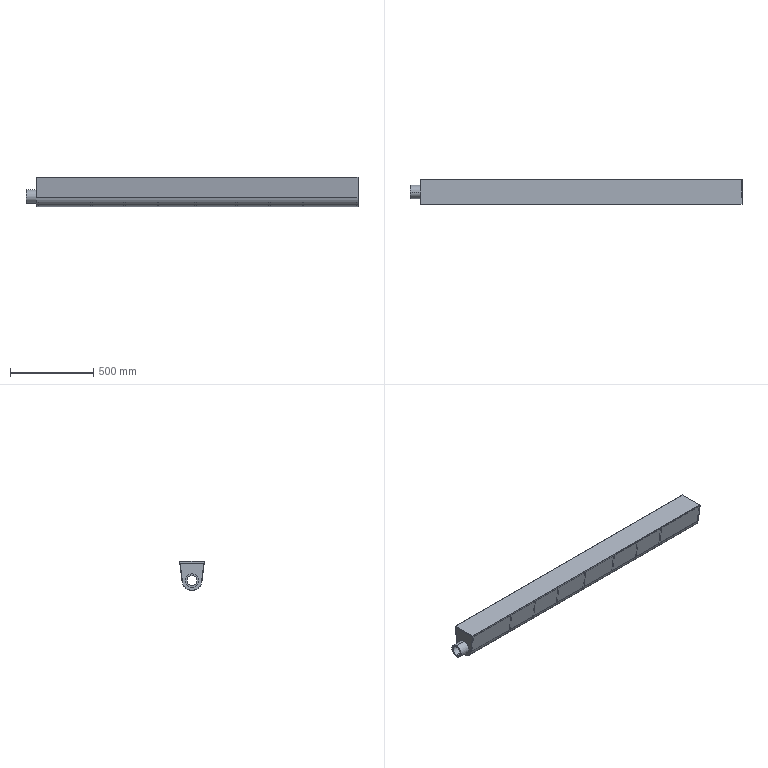Part | SolidWorks | features MirrorStock 1 | 12 solids | 100 faces | box 1995 x 150 x 175 mm | volume 10047262 mm3 | plane 61 | cylinder 39 | commonest cylinder face diameters 80 x20 116 x11 10 x4 60 x2 120 x2